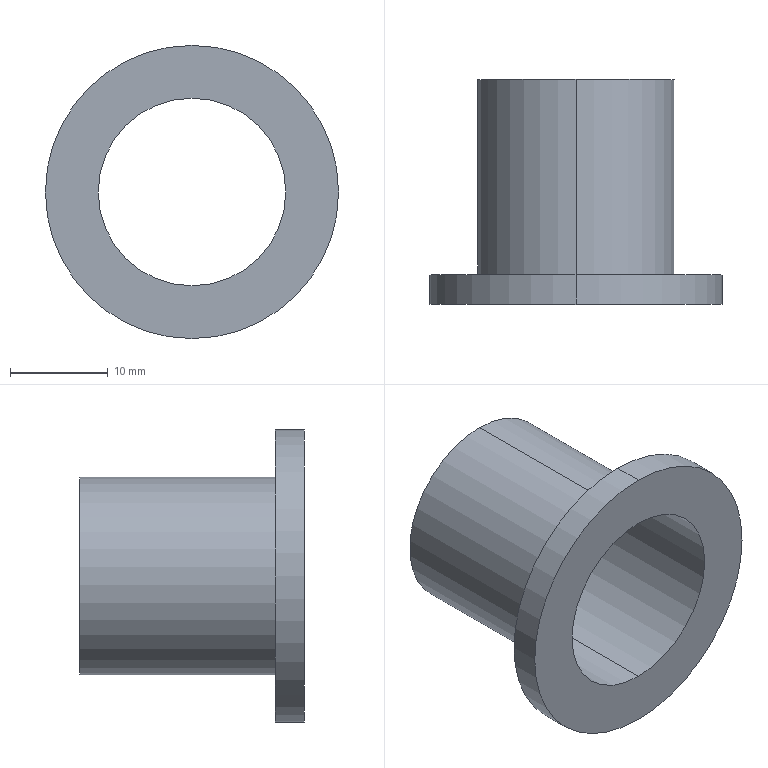Part | SolidWorks | features ICE 2, Extrusion 1 | 1 solid | 9 faces | box 30 x 23 x 30 mm | volume 1871 mm3 | cylinder 6 | plane 3 | commonest cylinder face diameters 19.2 x2 20.2 x2 30 x2
STEP:
#1=CARTESIAN_POINT('',(0.,-3.,-9.6));
#2=VERTEX_POINT('',#1);
#3=CARTESIAN_POINT('',(0.,-3.,9.6));
#4=VERTEX_POINT('',#3);
#5=CARTESIAN_POINT('',(0.,-3.,0.));
#6=DIRECTION('',(0.,1.,0.));
#7=DIRECTION('',(0.,0.,1.));
#8=AXIS2_PLACEMENT_3D('',#5,#6,#7);
#9=CIRCLE('',#8,9.6);
#10=EDGE_CURVE('',#2,#4,#9,.T.);
#11=ORIENTED_EDGE('',*,*,#10,.F.);
#12=CARTESIAN_POINT('',(0.,20.,-9.6));
#13=VERTEX_POINT('',#12);
#14=CARTESIAN_POINT('',(0.,-3.,-9.6));
#15=DIRECTION('',(0.,1.,0.));
#16=VECTOR('',#15,1000.);
#17=LINE('',#14,#16);
#18=EDGE_CURVE('',#2,#13,#17,.T.);
#19=ORIENTED_EDGE('',*,*,#18,.T.);
#20=CARTESIAN_POINT('',(0.,20.,9.6));
#21=VERTEX_POINT('',#20);
#22=CARTESIAN_POINT('',(0.,20.,0.));
#23=DIRECTION('',(0.,1.,0.));
#24=DIRECTION('',(0.,0.,1.));
#25=AXIS2_PLACEMENT_3D('',#22,#23,#24);
#26=CIRCLE('',#25,9.6);
#27=EDGE_CURVE('',#13,#21,#26,.T.);
#28=ORIENTED_EDGE('',*,*,#27,.T.);
#29=CARTESIAN_POINT('',(0.,-3.,9.6));
#30=DIRECTION('',(0.,1.,0.));
#31=VECTOR('',#30,1000.);
#32=LINE('',#29,#31);
#33=EDGE_CURVE('',#4,#21,#32,.T.);
#34=ORIENTED_EDGE('',*,*,#33,.F.);
#35=EDGE_LOOP('',(#11,#19,#28,#34));
#36=FACE_OUTER_BOUND('',#35,.T.);
#37=CARTESIAN_POINT('',(0.,-3.,0.));
#38=DIRECTION('',(0.,1.,0.));
#39=DIRECTION('',(0.,0.,1.));
#40=AXIS2_PLACEMENT_3D('',#37,#38,#39);
#41=CYLINDRICAL_SURFACE('',#40,9.6);
#42=ADVANCED_FACE('',(#36),#41,.F.);
#43=CARTESIAN_POINT('',(0.,0.,-15.));
#44=VERTEX_POINT('',#43);
#45=CARTESIAN_POINT('',(0.,0.,15.));
#46=VERTEX_POINT('',#45);
#47=CARTESIAN_POINT('',(0.,0.,0.));
#48=DIRECTION('',(0.,-1.,0.));
#49=DIRECTION('',(0.,0.,-1.));
#50=AXIS2_PLACEMENT_3D('',#47,#48,#49);
#51=CIRCLE('',#50,15.);
#52=EDGE_CURVE('',#44,#46,#51,.T.);
#53=ORIENTED_EDGE('',*,*,#52,.T.);
#54=CARTESIAN_POINT('',(0.,-3.,15.));
#55=VERTEX_POINT('',#54);
#56=CARTESIAN_POINT('',(0.,0.,15.));
#57=DIRECTION('',(0.,-1.,0.));
#58=VECTOR('',#57,1000.);
#59=LINE('',#56,#58);
#60=EDGE_CURVE('',#46,#55,#59,.T.);
#61=ORIENTED_EDGE('',*,*,#60,.T.);
#62=CARTESIAN_POINT('',(0.,-3.,-15.));
#63=VERTEX_POINT('',#62);
#64=CARTESIAN_POINT('',(0.,-3.,0.));
#65=DIRECTION('',(0.,-1.,0.));
#66=DIRECTION('',(0.,0.,-1.));
#67=AXIS2_PLACEMENT_3D('',#64,#65,#66);
#68=CIRCLE('',#67,15.);
#69=EDGE_CURVE('',#63,#55,#68,.T.);
#70=ORIENTED_EDGE('',*,*,#69,.F.);
#71=CARTESIAN_POINT('',(0.,0.,-15.));
#72=DIRECTION('',(0.,-1.,0.));
#73=VECTOR('',#72,1000.);
#74=LINE('',#71,#73);
#75=EDGE_CURVE('',#44,#63,#74,.T.);
#76=ORIENTED_EDGE('',*,*,#75,.F.);
#77=EDGE_LOOP('',(#53,#61,#70,#76));
#78=FACE_OUTER_BOUND('',#77,.T.);
#79=CARTESIAN_POINT('',(0.,0.,0.));
#80=DIRECTION('',(0.,-1.,0.));
#81=DIRECTION('',(0.,0.,-1.));
#82=AXIS2_PLACEMENT_3D('',#79,#80,#81);
#83=CYLINDRICAL_SURFACE('',#82,15.);
#84=ADVANCED_FACE('',(#78),#83,.T.);
#85=CARTESIAN_POINT('',(0.,20.,10.1));
#86=VERTEX_POINT('',#85);
#87=CARTESIAN_POINT('',(0.,20.,-10.1));
#88=VERTEX_POINT('',#87);
#89=CARTESIAN_POINT('',(0.,20.,0.));
#90=DIRECTION('',(0.,1.,0.));
#91=DIRECTION('',(0.,0.,1.));
#92=AXIS2_PLACEMENT_3D('',#89,#90,#91);
#93=CIRCLE('',#92,10.1);
#94=EDGE_CURVE('',#86,#88,#93,.T.);
#95=ORIENTED_EDGE('',*,*,#94,.F.);
#96=CARTESIAN_POINT('',(0.,0.,10.1));
#97=VERTEX_POINT('',#96);
#98=CARTESIAN_POINT('',(0.,20.,10.1));
#99=DIRECTION('',(0.,-1.,0.));
#100=VECTOR('',#99,1000.);
#101=LINE('',#98,#100);
#102=EDGE_CURVE('',#86,#97,#101,.T.);
#103=ORIENTED_EDGE('',*,*,#102,.T.);
#104=CARTESIAN_POINT('',(0.,0.,-10.1));
#105=VERTEX_POINT('',#104);
#106=CARTESIAN_POINT('',(0.,0.,0.));
#107=DIRECTION('',(0.,1.,0.));
#108=DIRECTION('',(0.,0.,1.));
#109=AXIS2_PLACEMENT_3D('',#106,#107,#108);
#110=CIRCLE('',#109,10.1);
#111=EDGE_CURVE('',#97,#105,#110,.T.);
#112=ORIENTED_EDGE('',*,*,#111,.T.);
#113=CARTESIAN_POINT('',(0.,20.,-10.1));
#114=DIRECTION('',(0.,-1.,0.));
#115=VECTOR('',#114,1000.);
#116=LINE('',#113,#115);
#117=EDGE_CURVE('',#88,#105,#116,.T.);
#118=ORIENTED_EDGE('',*,*,#117,.F.);
#119=EDGE_LOOP('',(#95,#103,#112,#118));
#120=FACE_OUTER_BOUND('',#119,.T.);
#121=CARTESIAN_POINT('',(0.,20.,0.));
#122=DIRECTION('',(0.,-1.,0.));
#123=DIRECTION('',(0.,0.,-1.));
#124=AXIS2_PLACEMENT_3D('',#121,#122,#123);
#125=CYLINDRICAL_SURFACE('',#124,10.1);
#126=ADVANCED_FACE('',(#120),#125,.T.);
#127=ORIENTED_EDGE('',*,*,#102,.F.);
#128=CARTESIAN_POINT('',(0.,20.,0.));
#129=DIRECTION('',(0.,1.,0.));
#130=DIRECTION('',(0.,0.,1.));
#131=AXIS2_PLACEMENT_3D('',#128,#129,#130);
#132=CIRCLE('',#131,10.1);
#133=EDGE_CURVE('',#88,#86,#132,.T.);
#134=ORIENTED_EDGE('',*,*,#133,.F.);
#135=ORIENTED_EDGE('',*,*,#117,.T.);
#136=CARTESIAN_POINT('',(0.,0.,0.));
#137=DIRECTION('',(0.,1.,0.));
#138=DIRECTION('',(0.,0.,1.));
#139=AXIS2_PLACEMENT_3D('',#136,#137,#138);
#140=CIRCLE('',#139,10.1);
#141=EDGE_CURVE('',#105,#97,#140,.T.);
#142=ORIENTED_EDGE('',*,*,#141,.T.);
#143=EDGE_LOOP('',(#127,#134,#135,#142));
#144=FACE_OUTER_BOUND('',#143,.T.);
#145=CARTESIAN_POINT('',(0.,20.,0.));
#146=DIRECTION('',(0.,-1.,0.));
#147=DIRECTION('',(0.,0.,-1.));
#148=AXIS2_PLACEMENT_3D('',#145,#146,#147);
#149=CYLINDRICAL_SURFACE('',#148,10.1);
#150=ADVANCED_FACE('',(#144),#149,.T.);
#151=CARTESIAN_POINT('',(0.,20.,0.));
#152=DIRECTION('',(0.,1.,0.));
#153=DIRECTION('',(0.,0.,1.));
#154=AXIS2_PLACEMENT_3D('',#151,#152,#153);
#155=CIRCLE('',#154,9.6);
#156=EDGE_CURVE('',#21,#13,#155,.T.);
#157=ORIENTED_EDGE('',*,*,#156,.F.);
#158=ORIENTED_EDGE('',*,*,#27,.F.);
#159=EDGE_LOOP('',(#157,#158));
#160=FACE_BOUND('',#159,.T.);
#161=ORIENTED_EDGE('',*,*,#133,.T.);
#162=ORIENTED_EDGE('',*,*,#94,.T.);
#163=EDGE_LOOP('',(#161,#162));
#164=FACE_OUTER_BOUND('',#163,.T.);
#165=CARTESIAN_POINT('',(0.,20.,0.));
#166=DIRECTION('',(0.,1.,0.));
#167=DIRECTION('',(0.,0.,1.));
#168=AXIS2_PLACEMENT_3D('',#165,#166,#167);
#169=PLANE('',#168);
#170=ADVANCED_FACE('',(#160,#164),#169,.T.);
#171=ORIENTED_EDGE('',*,*,#60,.F.);
#172=CARTESIAN_POINT('',(0.,0.,0.));
#173=DIRECTION('',(0.,-1.,0.));
#174=DIRECTION('',(0.,0.,-1.));
#175=AXIS2_PLACEMENT_3D('',#172,#173,#174);
#176=CIRCLE('',#175,15.);
#177=EDGE_CURVE('',#46,#44,#176,.T.);
#178=ORIENTED_EDGE('',*,*,#177,.T.);
#179=ORIENTED_EDGE('',*,*,#75,.T.);
#180=CARTESIAN_POINT('',(0.,-3.,0.));
#181=DIRECTION('',(0.,-1.,0.));
#182=DIRECTION('',(0.,0.,-1.));
#183=AXIS2_PLACEMENT_3D('',#180,#181,#182);
#184=CIRCLE('',#183,15.);
#185=EDGE_CURVE('',#55,#63,#184,.T.);
#186=ORIENTED_EDGE('',*,*,#185,.F.);
#187=EDGE_LOOP('',(#171,#178,#179,#186));
#188=FACE_OUTER_BOUND('',#187,.T.);
#189=CARTESIAN_POINT('',(0.,0.,0.));
#190=DIRECTION('',(0.,-1.,0.));
#191=DIRECTION('',(0.,0.,-1.));
#192=AXIS2_PLACEMENT_3D('',#189,#190,#191);
#193=CYLINDRICAL_SURFACE('',#192,15.);
#194=ADVANCED_FACE('',(#188),#193,.T.);
#195=ORIENTED_EDGE('',*,*,#141,.F.);
#196=ORIENTED_EDGE('',*,*,#111,.F.);
#197=EDGE_LOOP('',(#195,#196));
#198=FACE_BOUND('',#197,.T.);
#199=ORIENTED_EDGE('',*,*,#52,.F.);
#200=ORIENTED_EDGE('',*,*,#177,.F.);
#201=EDGE_LOOP('',(#199,#200));
#202=FACE_OUTER_BOUND('',#201,.T.);
#203=CARTESIAN_POINT('',(0.,0.,0.));
#204=DIRECTION('',(0.,-1.,0.));
#205=DIRECTION('',(0.,0.,-1.));
#206=AXIS2_PLACEMENT_3D('',#203,#204,#205);
#207=PLANE('',#206);
#208=ADVANCED_FACE('',(#198,#202),#207,.F.);
#209=CARTESIAN_POINT('',(0.,-3.,0.));
#210=DIRECTION('',(0.,1.,0.));
#211=DIRECTION('',(0.,0.,1.));
#212=AXIS2_PLACEMENT_3D('',#209,#210,#211);
#213=CIRCLE('',#212,9.6);
#214=EDGE_CURVE('',#4,#2,#213,.T.);
#215=ORIENTED_EDGE('',*,*,#214,.T.);
#216=ORIENTED_EDGE('',*,*,#10,.T.);
#217=EDGE_LOOP('',(#215,#216));
#218=FACE_BOUND('',#217,.T.);
#219=ORIENTED_EDGE('',*,*,#69,.T.);
#220=ORIENTED_EDGE('',*,*,#185,.T.);
#221=EDGE_LOOP('',(#219,#220));
#222=FACE_OUTER_BOUND('',#221,.T.);
#223=CARTESIAN_POINT('',(0.,-3.,0.));
#224=DIRECTION('',(0.,-1.,0.));
#225=DIRECTION('',(0.,0.,-1.));
#226=AXIS2_PLACEMENT_3D('',#223,#224,#225);
#227=PLANE('',#226);
#228=ADVANCED_FACE('',(#218,#222),#227,.T.);
#229=ORIENTED_EDGE('',*,*,#18,.F.);
#230=ORIENTED_EDGE('',*,*,#214,.F.);
#231=ORIENTED_EDGE('',*,*,#33,.T.);
#232=ORIENTED_EDGE('',*,*,#156,.T.);
#233=EDGE_LOOP('',(#229,#230,#231,#232));
#234=FACE_OUTER_BOUND('',#233,.T.);
#235=CARTESIAN_POINT('',(0.,-3.,0.));
#236=DIRECTION('',(0.,1.,0.));
#237=DIRECTION('',(0.,0.,1.));
#238=AXIS2_PLACEMENT_3D('',#235,#236,#237);
#239=CYLINDRICAL_SURFACE('',#238,9.6);
#240=ADVANCED_FACE('',(#234),#239,.F.);
#241=CLOSED_SHELL('',(#42,#84,#126,#150,#170,#194,#208,#228,#240));
#242=MANIFOLD_SOLID_BREP('',#241);
#243=CARTESIAN_POINT('',(0.,0.,0.));
#244=DIRECTION('',(0.,0.,1.));
#245=DIRECTION('',(1.,0.,0.));
#246=AXIS2_PLACEMENT_3D('',#243,#244,#245);
#247=(LENGTH_UNIT()NAMED_UNIT(*)SI_UNIT(.MILLI.,.METRE.));
#248=UNCERTAINTY_MEASURE_WITH_UNIT(LENGTH_MEASURE(0.00001),#247,'','');
#249=(NAMED_UNIT(*)PLANE_ANGLE_UNIT()SI_UNIT($,.RADIAN.));
#250=(NAMED_UNIT(*)SI_UNIT($,.STERADIAN.)SOLID_ANGLE_UNIT());
#251=(GEOMETRIC_REPRESENTATION_CONTEXT(3)GLOBAL_UNCERTAINTY_ASSIGNED_CONTEXT((#248))GLOBAL_UNIT_ASSIGNED_CONTEXT((#247,#249,#250))REPRESENTATION_CONTEXT('',''));
#252=ADVANCED_BREP_SHAPE_REPRESENTATION('',(#242,#246),#251);